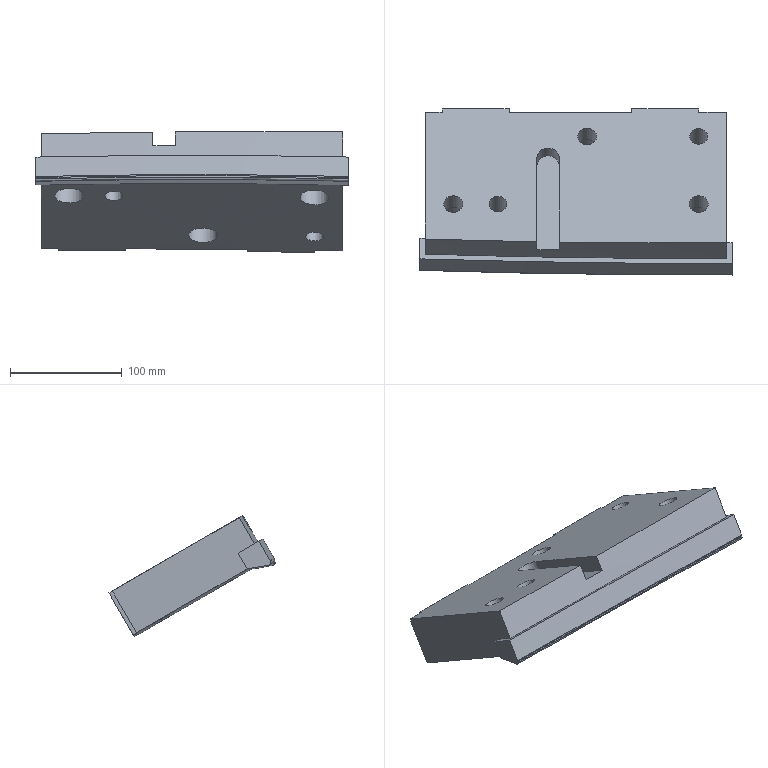Part | NX | features MAIN_BODY 2 | 1 solid | 39 faces | box 280 x 148.918 x 108.36 mm | volume 1561277 mm3 | plane 22 | cylinder 9 | spline 8 | commonest cylinder face diameters 17 x3 26 x3 16 x2 20 x1